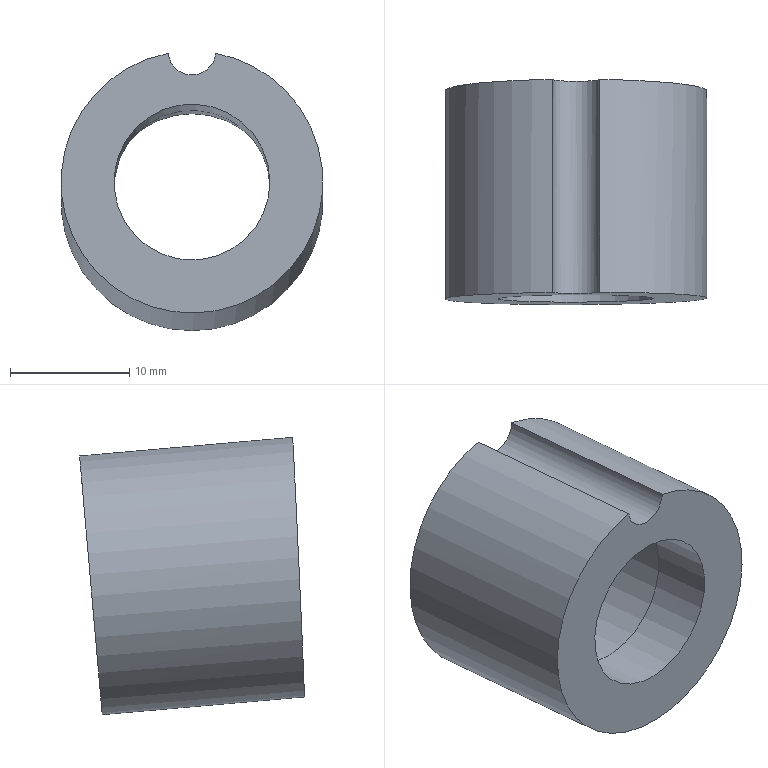Part | NX | features EKSD 22-20-13.10 2 | 1 solid | 7 faces | box 22 x 18.889 x 23.301 mm | volume 3796 mm3 | cylinder 4 | plane 3 | commonest cylinder face diameters 4 x1 13.1 x1 14.6 x1 22 x1
STEP:
#1=CARTESIAN_POINT('',(-122.444,-28.021,-27.736));
#2=VERTEX_POINT('',#1);
#3=CARTESIAN_POINT('',(-118.461,-28.021,-27.736));
#4=VERTEX_POINT('',#3);
#5=CARTESIAN_POINT('',(-120.452,-28.005,-27.555));
#6=DIRECTION('',(0.,-0.9962,0.08716));
#7=DIRECTION('',(0.,-0.08716,-0.9962));
#8=AXIS2_PLACEMENT_3D('',#5,#6,#7);
#9=CIRCLE('',#8,2.);
#10=EDGE_CURVE('',#2,#4,#9,.T.);
#11=ORIENTED_EDGE('',*,*,#10,.T.);
#12=CARTESIAN_POINT('',(-120.452,-28.964,-38.513));
#13=DIRECTION('',(0.,-0.9962,0.08716));
#14=DIRECTION('',(0.,-0.08716,-0.9962));
#15=AXIS2_PLACEMENT_3D('',#12,#13,#14);
#16=CIRCLE('',#15,11.);
#17=EDGE_CURVE('',#2,#4,#16,.T.);
#18=ORIENTED_EDGE('',*,*,#17,.F.);
#19=EDGE_LOOP('',(#11,#18));
#20=FACE_BOUND('',#19,.T.);
#21=CARTESIAN_POINT('',(-120.452,-28.327,-31.241));
#22=VERTEX_POINT('',#21);
#23=CARTESIAN_POINT('',(-120.452,-28.964,-38.513));
#24=DIRECTION('',(0.,0.9962,-0.08716));
#25=DIRECTION('',(0.,0.08716,0.9962));
#26=AXIS2_PLACEMENT_3D('',#23,#24,#25);
#27=CIRCLE('',#26,7.3);
#28=EDGE_CURVE('',#22,#22,#27,.T.);
#29=ORIENTED_EDGE('',*,*,#28,.F.);
#30=EDGE_LOOP('',(#29));
#31=FACE_BOUND('',#30,.T.);
#32=CARTESIAN_POINT('',(-120.452,-28.964,-38.513));
#33=DIRECTION('',(0.,0.9962,-0.08716));
#34=DIRECTION('',(0.,0.08716,0.9962));
#35=AXIS2_PLACEMENT_3D('',#32,#33,#34);
#36=PLANE('',#35);
#37=ADVANCED_FACE('',(#20,#31),#36,.T.);
#38=CARTESIAN_POINT('',(-118.461,-45.907,-26.171));
#39=VERTEX_POINT('',#38);
#40=CARTESIAN_POINT('',(-122.444,-45.922,-26.17));
#41=VERTEX_POINT('',#40);
#42=CARTESIAN_POINT('',(-120.452,-45.906,-25.989));
#43=DIRECTION('',(0.00391,-0.999,0.04549));
#44=DIRECTION('',(0.09317,-0.04493,-0.9946));
#45=AXIS2_PLACEMENT_3D('',#42,#43,#44);
#46=ELLIPSE('',#45,2.002,2.);
#47=EDGE_CURVE('',#39,#41,#46,.F.);
#48=ORIENTED_EDGE('',*,*,#47,.T.);
#49=CARTESIAN_POINT('',(-120.452,-46.407,-36.987));
#50=DIRECTION('',(0.00391,-0.999,0.04549));
#51=DIRECTION('',(0.09317,-0.04493,-0.9946));
#52=AXIS2_PLACEMENT_3D('',#49,#50,#51);
#53=ELLIPSE('',#52,11.01,11.);
#54=EDGE_CURVE('',#39,#41,#53,.F.);
#55=ORIENTED_EDGE('',*,*,#54,.F.);
#56=EDGE_LOOP('',(#48,#55));
#57=FACE_BOUND('',#56,.T.);
#58=CARTESIAN_POINT('',(-119.842,-46.702,-43.508));
#59=VERTEX_POINT('',#58);
#60=CARTESIAN_POINT('',(-120.452,-46.407,-36.987));
#61=DIRECTION('',(0.00391,-0.999,0.04549));
#62=DIRECTION('',(0.09317,-0.04493,-0.9946));
#63=AXIS2_PLACEMENT_3D('',#60,#61,#62);
#64=ELLIPSE('',#63,6.556,6.55);
#65=EDGE_CURVE('',#59,#59,#64,.T.);
#66=ORIENTED_EDGE('',*,*,#65,.F.);
#67=EDGE_LOOP('',(#66));
#68=FACE_BOUND('',#67,.T.);
#69=CARTESIAN_POINT('',(-78.701,-48.763,-92.296));
#70=DIRECTION('',(0.00391,-0.999,0.04549));
#71=DIRECTION('',(-0.05224,0.04523,0.9976));
#72=AXIS2_PLACEMENT_3D('',#69,#70,#71);
#73=PLANE('',#72);
#74=ADVANCED_FACE('',(#57,#68),#73,.T.);
#75=CARTESIAN_POINT('',(-118.461,-37.983,-26.865));
#76=DIRECTION('',(0.,0.9962,-0.08716));
#77=VECTOR('',#76,1000.);
#78=LINE('',#75,#77);
#79=EDGE_CURVE('',#39,#4,#78,.T.);
#80=ORIENTED_EDGE('',*,*,#79,.F.);
#81=ORIENTED_EDGE('',*,*,#54,.T.);
#82=CARTESIAN_POINT('',(-122.444,-37.983,-26.865));
#83=DIRECTION('',(0.,0.9962,-0.08716));
#84=VECTOR('',#83,1000.);
#85=LINE('',#82,#84);
#86=EDGE_CURVE('',#2,#41,#85,.F.);
#87=ORIENTED_EDGE('',*,*,#86,.F.);
#88=ORIENTED_EDGE('',*,*,#17,.T.);
#89=EDGE_LOOP('',(#80,#81,#87,#88));
#90=FACE_BOUND('',#89,.T.);
#91=CARTESIAN_POINT('',(-120.452,-48.887,-36.77));
#92=DIRECTION('',(0.,0.9962,-0.08716));
#93=DIRECTION('',(0.,0.08716,0.9962));
#94=AXIS2_PLACEMENT_3D('',#91,#92,#93);
#95=CYLINDRICAL_SURFACE('',#94,11.);
#96=ADVANCED_FACE('',(#90),#95,.T.);
#97=CARTESIAN_POINT('',(-120.452,-41.489,-43.992));
#98=VERTEX_POINT('',#97);
#99=CARTESIAN_POINT('',(-120.452,-40.918,-37.467));
#100=DIRECTION('',(0.,-0.9962,0.08716));
#101=DIRECTION('',(0.,-0.08716,-0.9962));
#102=AXIS2_PLACEMENT_3D('',#99,#100,#101);
#103=CIRCLE('',#102,6.55);
#104=EDGE_CURVE('',#98,#98,#103,.F.);
#105=ORIENTED_EDGE('',*,*,#104,.T.);
#106=EDGE_LOOP('',(#105));
#107=FACE_BOUND('',#106,.T.);
#108=ORIENTED_EDGE('',*,*,#65,.T.);
#109=EDGE_LOOP('',(#108));
#110=FACE_BOUND('',#109,.T.);
#111=CARTESIAN_POINT('',(-120.452,-49.884,-36.683));
#112=DIRECTION('',(0.,0.9962,-0.08716));
#113=DIRECTION('',(0.,0.08716,0.9962));
#114=AXIS2_PLACEMENT_3D('',#111,#112,#113);
#115=CYLINDRICAL_SURFACE('',#114,6.55);
#116=ADVANCED_FACE('',(#107,#110),#115,.F.);
#117=CARTESIAN_POINT('',(-120.452,-40.282,-30.195));
#118=VERTEX_POINT('',#117);
#119=CARTESIAN_POINT('',(-120.452,-40.918,-37.467));
#120=DIRECTION('',(0.,0.9962,-0.08716));
#121=DIRECTION('',(0.,0.08716,0.9962));
#122=AXIS2_PLACEMENT_3D('',#119,#120,#121);
#123=CIRCLE('',#122,7.3);
#124=EDGE_CURVE('',#118,#118,#123,.T.);
#125=ORIENTED_EDGE('',*,*,#124,.T.);
#126=EDGE_LOOP('',(#125));
#127=FACE_BOUND('',#126,.T.);
#128=ORIENTED_EDGE('',*,*,#104,.F.);
#129=EDGE_LOOP('',(#128));
#130=FACE_BOUND('',#129,.T.);
#131=CARTESIAN_POINT('',(-120.452,-40.918,-37.467));
#132=DIRECTION('',(0.,-0.9962,0.08716));
#133=DIRECTION('',(0.,-0.08716,-0.9962));
#134=AXIS2_PLACEMENT_3D('',#131,#132,#133);
#135=PLANE('',#134);
#136=ADVANCED_FACE('',(#127,#130),#135,.F.);
#137=ORIENTED_EDGE('',*,*,#28,.T.);
#138=EDGE_LOOP('',(#137));
#139=FACE_BOUND('',#138,.T.);
#140=ORIENTED_EDGE('',*,*,#124,.F.);
#141=EDGE_LOOP('',(#140));
#142=FACE_BOUND('',#141,.T.);
#143=CARTESIAN_POINT('',(-120.452,-40.918,-37.467));
#144=DIRECTION('',(0.,0.9962,-0.08716));
#145=DIRECTION('',(0.,0.08716,0.9962));
#146=AXIS2_PLACEMENT_3D('',#143,#144,#145);
#147=CYLINDRICAL_SURFACE('',#146,7.3);
#148=ADVANCED_FACE('',(#139,#142),#147,.F.);
#149=ORIENTED_EDGE('',*,*,#79,.T.);
#150=ORIENTED_EDGE('',*,*,#10,.F.);
#151=ORIENTED_EDGE('',*,*,#86,.T.);
#152=ORIENTED_EDGE('',*,*,#47,.F.);
#153=EDGE_LOOP('',(#149,#150,#151,#152));
#154=FACE_BOUND('',#153,.T.);
#155=CARTESIAN_POINT('',(-120.452,-47.929,-25.812));
#156=DIRECTION('',(0.,0.9962,-0.08716));
#157=DIRECTION('',(0.,0.08716,0.9962));
#158=AXIS2_PLACEMENT_3D('',#155,#156,#157);
#159=CYLINDRICAL_SURFACE('',#158,2.);
#160=ADVANCED_FACE('',(#154),#159,.F.);
#161=CLOSED_SHELL('',(#37,#74,#96,#116,#136,#148,#160));
#162=MANIFOLD_SOLID_BREP('',#161);
#163=(LENGTH_UNIT()NAMED_UNIT(*)SI_UNIT(.MILLI.,.METRE.));
#164=UNCERTAINTY_MEASURE_WITH_UNIT(LENGTH_MEASURE(0.00001),#163,'','');
#165=(NAMED_UNIT(*)PLANE_ANGLE_UNIT()SI_UNIT($,.RADIAN.));
#166=(NAMED_UNIT(*)SI_UNIT($,.STERADIAN.)SOLID_ANGLE_UNIT());
#167=(GEOMETRIC_REPRESENTATION_CONTEXT(3)GLOBAL_UNCERTAINTY_ASSIGNED_CONTEXT((#164))GLOBAL_UNIT_ASSIGNED_CONTEXT((#163,#165,#166))REPRESENTATION_CONTEXT('',''));
#168=ADVANCED_BREP_SHAPE_REPRESENTATION('',(#162),#167);